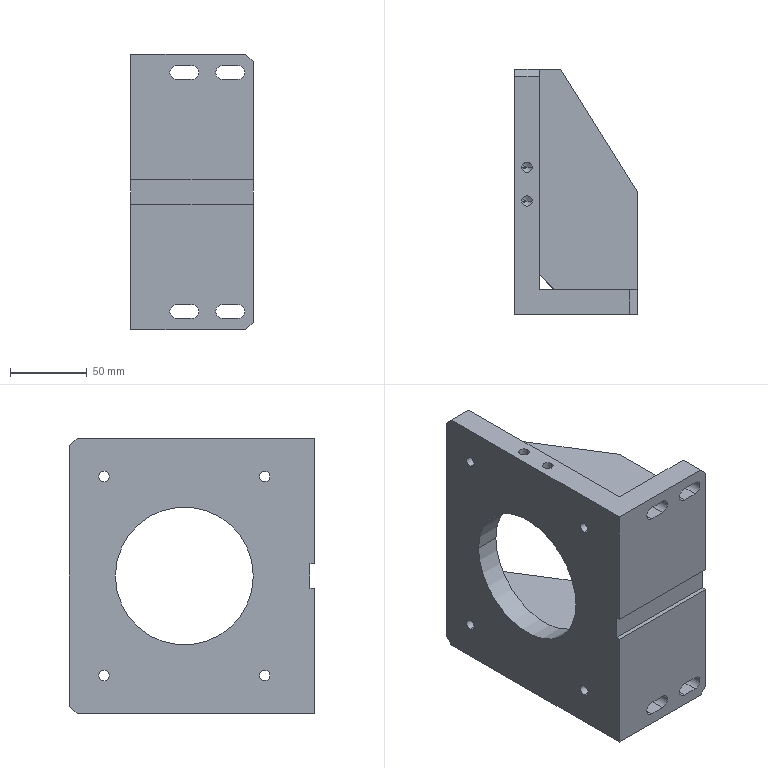Part | STEP file | PN_0017 Motor BKT_Default | 3 solids | 82 faces | box 80 x 160 x 180 mm | volume 722805 mm3 | plane 40 | cylinder 30 | cone 12 | commonest cylinder face diameters 6.8 x20 9 x8 90 x2